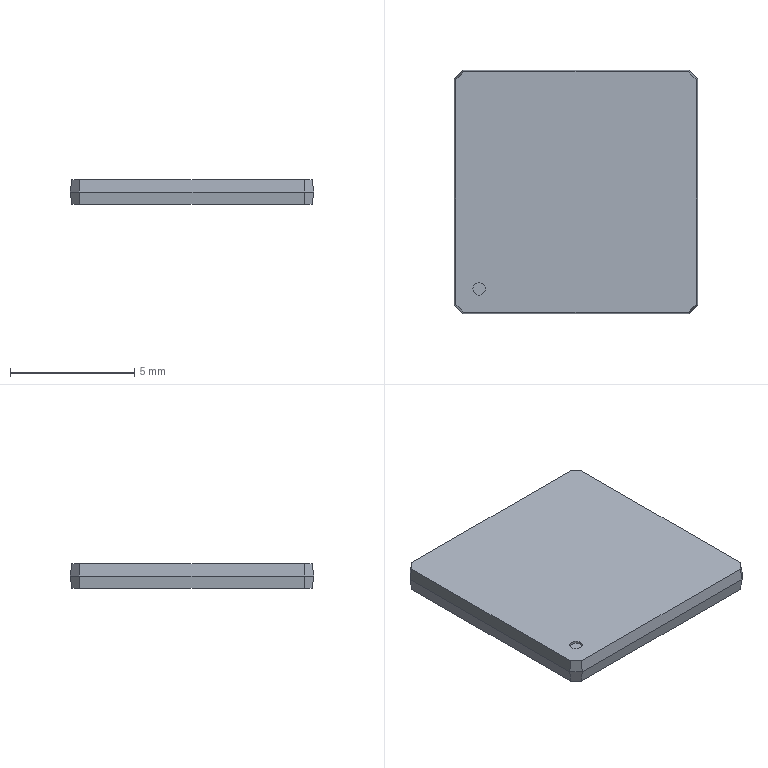Part | STEP file | RJ-USIO-V1_2-220411_260 | 1 solid | 21 faces | box 9.8 x 9.8 x 1 mm | volume 94.601 mm3 | plane 19 | cylinder 2 | commonest cylinder face diameters 0.5 x2
STEP:
#1=CARTESIAN_POINT('',(0.,0.,0.));
#2=DIRECTION('',(0.,0.,1.));
#3=DIRECTION('',(1.,0.,0.));
#4=AXIS2_PLACEMENT_3D('',#1,#2,#3);
#5=CARTESIAN_POINT('',(46.95,46.8,0.9));
#6=VERTEX_POINT('',#5);
#7=CARTESIAN_POINT('',(46.45,46.8,0.9));
#8=VERTEX_POINT('',#7);
#9=CARTESIAN_POINT('',(46.7,46.8,0.9));
#10=DIRECTION('',(0.,0.,1.));
#11=DIRECTION('',(1.,0.,0.));
#12=AXIS2_PLACEMENT_3D('',#9,#10,#11);
#13=CIRCLE('',#12,0.25);
#14=CARTESIAN_POINT('',(46.7,46.8,0.9));
#15=DIRECTION('',(0.,0.,1.));
#16=DIRECTION('',(-1.,0.,0.));
#17=AXIS2_PLACEMENT_3D('',#14,#15,#16);
#18=PLANE('',#17);
#19=CARTESIAN_POINT('',(0.,0.));
#20=DIRECTION('',(-1.,0.));
#21=AXIS2_PLACEMENT_2D('',#19,#20);
#22=CIRCLE('',#21,0.25);
#23=(GEOMETRIC_REPRESENTATION_CONTEXT(2)PARAMETRIC_REPRESENTATION_CONTEXT()REPRESENTATION_CONTEXT('',''));
#24=DEFINITIONAL_REPRESENTATION('',(#22),#23);
#25=PCURVE('',#18,#24);
#26=CARTESIAN_POINT('',(46.7,46.8,0.9));
#27=DIRECTION('',(0.,0.,1.));
#28=DIRECTION('',(-1.,0.,0.));
#29=AXIS2_PLACEMENT_3D('',#26,#27,#28);
#30=CYLINDRICAL_SURFACE('',#29,0.25);
#31=CARTESIAN_POINT('',(3.142,0.));
#32=DIRECTION('',(1.,0.));
#33=VECTOR('',#32,1.);
#34=LINE('',#31,#33);
#35=(GEOMETRIC_REPRESENTATION_CONTEXT(2)PARAMETRIC_REPRESENTATION_CONTEXT()REPRESENTATION_CONTEXT('',''));
#36=DEFINITIONAL_REPRESENTATION('',(#34),#35);
#37=PCURVE('',#30,#36);
#38=SURFACE_CURVE('',#13,(#25,#37),.PCURVE_S1.);
#39=EDGE_CURVE('',#6,#8,#38,.T.);
#40=ORIENTED_EDGE('',*,*,#39,.F.);
#41=CARTESIAN_POINT('',(46.7,46.8,0.9));
#42=DIRECTION('',(0.,0.,1.));
#43=DIRECTION('',(-1.,0.,0.));
#44=AXIS2_PLACEMENT_3D('',#41,#42,#43);
#45=CIRCLE('',#44,0.25);
#46=CARTESIAN_POINT('',(0.,0.));
#47=DIRECTION('',(1.,0.));
#48=AXIS2_PLACEMENT_2D('',#46,#47);
#49=CIRCLE('',#48,0.25);
#50=(GEOMETRIC_REPRESENTATION_CONTEXT(2)PARAMETRIC_REPRESENTATION_CONTEXT()REPRESENTATION_CONTEXT('',''));
#51=DEFINITIONAL_REPRESENTATION('',(#49),#50);
#52=PCURVE('',#18,#51);
#53=CARTESIAN_POINT('',(46.7,46.8,0.9));
#54=DIRECTION('',(0.,0.,1.));
#55=DIRECTION('',(-1.,0.,0.));
#56=AXIS2_PLACEMENT_3D('',#53,#54,#55);
#57=CYLINDRICAL_SURFACE('',#56,0.25);
#58=CARTESIAN_POINT('',(0.,0.));
#59=DIRECTION('',(1.,0.));
#60=VECTOR('',#59,1.);
#61=LINE('',#58,#60);
#62=(GEOMETRIC_REPRESENTATION_CONTEXT(2)PARAMETRIC_REPRESENTATION_CONTEXT()REPRESENTATION_CONTEXT('',''));
#63=DEFINITIONAL_REPRESENTATION('',(#61),#62);
#64=PCURVE('',#57,#63);
#65=SURFACE_CURVE('',#45,(#52,#64),.PCURVE_S1.);
#66=EDGE_CURVE('',#8,#6,#65,.T.);
#67=ORIENTED_EDGE('',*,*,#66,.F.);
#68=EDGE_LOOP('',(#40,#67));
#69=FACE_BOUND('',#68,.F.);
#70=ADVANCED_FACE('',(#69),#18,.T.);
#71=CARTESIAN_POINT('',(46.45,46.8,1.));
#72=VERTEX_POINT('',#71);
#73=CARTESIAN_POINT('',(46.45,46.8,0.9));
#74=DIRECTION('',(0.,0.,1.));
#75=VECTOR('',#74,1.);
#76=LINE('',#73,#75);
#77=CARTESIAN_POINT('',(6.283,0.));
#78=DIRECTION('',(0.,1.));
#79=VECTOR('',#78,1.);
#80=LINE('',#77,#79);
#81=(GEOMETRIC_REPRESENTATION_CONTEXT(2)PARAMETRIC_REPRESENTATION_CONTEXT()REPRESENTATION_CONTEXT('',''));
#82=DEFINITIONAL_REPRESENTATION('',(#80),#81);
#83=PCURVE('',#30,#82);
#84=CARTESIAN_POINT('',(0.,0.));
#85=DIRECTION('',(0.,1.));
#86=VECTOR('',#85,1.);
#87=LINE('',#84,#86);
#88=(GEOMETRIC_REPRESENTATION_CONTEXT(2)PARAMETRIC_REPRESENTATION_CONTEXT()REPRESENTATION_CONTEXT('',''));
#89=DEFINITIONAL_REPRESENTATION('',(#87),#88);
#90=PCURVE('',#57,#89);
#91=SURFACE_CURVE('',#76,(#83,#90),.PCURVE_S1.);
#92=EDGE_CURVE('',#8,#72,#91,.T.);
#93=ORIENTED_EDGE('',*,*,#92,.T.);
#94=CARTESIAN_POINT('',(46.95,46.8,1.));
#95=VERTEX_POINT('',#94);
#96=CARTESIAN_POINT('',(46.7,46.8,1.));
#97=DIRECTION('',(0.,0.,-1.));
#98=DIRECTION('',(-1.,0.,0.));
#99=AXIS2_PLACEMENT_3D('',#96,#97,#98);
#100=CIRCLE('',#99,0.25);
#101=CARTESIAN_POINT('',(6.283,0.1));
#102=DIRECTION('',(-1.,0.));
#103=VECTOR('',#102,1.);
#104=LINE('',#101,#103);
#105=(GEOMETRIC_REPRESENTATION_CONTEXT(2)PARAMETRIC_REPRESENTATION_CONTEXT()REPRESENTATION_CONTEXT('',''));
#106=DEFINITIONAL_REPRESENTATION('',(#104),#105);
#107=PCURVE('',#30,#106);
#108=CARTESIAN_POINT('',(45.7,45.8,1.));
#109=DIRECTION('',(0.,0.,1.));
#110=DIRECTION('',(-1.,0.,0.));
#111=AXIS2_PLACEMENT_3D('',#108,#109,#110);
#112=PLANE('',#111);
#113=CARTESIAN_POINT('',(-0.75,-1.));
#114=CARTESIAN_POINT('',(-0.75,-1.433));
#115=CARTESIAN_POINT('',(-1.125,-1.217));
#116=CARTESIAN_POINT('',(-1.5,-1.));
#117=CARTESIAN_POINT('',(-1.125,-0.7835));
#118=CARTESIAN_POINT('',(-0.75,-0.567));
#119=CARTESIAN_POINT('',(-0.75,-1.));
#120=(BOUNDED_CURVE()B_SPLINE_CURVE(2,(#113,#114,#115,#116,#117,#118,#119),.UNSPECIFIED.,.T.,.F.)B_SPLINE_CURVE_WITH_KNOTS((1,2,2,2,2,1),(-2.094,0.,2.094,4.189,6.283,8.378),.UNSPECIFIED.)CURVE()GEOMETRIC_REPRESENTATION_ITEM()RATIONAL_B_SPLINE_CURVE((1.,0.5,1.,0.5,1.,0.5,1.))REPRESENTATION_ITEM(''));
#121=(GEOMETRIC_REPRESENTATION_CONTEXT(2)PARAMETRIC_REPRESENTATION_CONTEXT()REPRESENTATION_CONTEXT('',''));
#122=DEFINITIONAL_REPRESENTATION('',(#120),#121);
#123=PCURVE('',#112,#122);
#124=SURFACE_CURVE('',#100,(#107,#123),.PCURVE_S1.);
#125=EDGE_CURVE('',#72,#95,#124,.T.);
#126=ORIENTED_EDGE('',*,*,#125,.T.);
#127=CARTESIAN_POINT('',(46.95,46.8,0.9));
#128=DIRECTION('',(0.,0.,1.));
#129=VECTOR('',#128,1.);
#130=LINE('',#127,#129);
#131=CARTESIAN_POINT('',(3.142,0.));
#132=DIRECTION('',(0.,1.));
#133=VECTOR('',#132,1.);
#134=LINE('',#131,#133);
#135=(GEOMETRIC_REPRESENTATION_CONTEXT(2)PARAMETRIC_REPRESENTATION_CONTEXT()REPRESENTATION_CONTEXT('',''));
#136=DEFINITIONAL_REPRESENTATION('',(#134),#135);
#137=PCURVE('',#30,#136);
#138=CARTESIAN_POINT('',(3.142,0.));
#139=DIRECTION('',(0.,1.));
#140=VECTOR('',#139,1.);
#141=LINE('',#138,#140);
#142=(GEOMETRIC_REPRESENTATION_CONTEXT(2)PARAMETRIC_REPRESENTATION_CONTEXT()REPRESENTATION_CONTEXT('',''));
#143=DEFINITIONAL_REPRESENTATION('',(#141),#142);
#144=PCURVE('',#57,#143);
#145=SURFACE_CURVE('',#130,(#137,#144),.PCURVE_S1.);
#146=EDGE_CURVE('',#6,#95,#145,.T.);
#147=ORIENTED_EDGE('',*,*,#146,.F.);
#148=ORIENTED_EDGE('',*,*,#39,.T.);
#149=EDGE_LOOP('',(#93,#126,#147,#148));
#150=FACE_BOUND('',#149,.F.);
#151=ADVANCED_FACE('',(#150),#30,.F.);
#152=ORIENTED_EDGE('',*,*,#66,.T.);
#153=ORIENTED_EDGE('',*,*,#146,.T.);
#154=CARTESIAN_POINT('',(46.7,46.8,1.));
#155=DIRECTION('',(0.,0.,-1.));
#156=DIRECTION('',(1.,0.,0.));
#157=AXIS2_PLACEMENT_3D('',#154,#155,#156);
#158=CIRCLE('',#157,0.25);
#159=CARTESIAN_POINT('',(3.142,0.1));
#160=DIRECTION('',(-1.,0.));
#161=VECTOR('',#160,1.);
#162=LINE('',#159,#161);
#163=(GEOMETRIC_REPRESENTATION_CONTEXT(2)PARAMETRIC_REPRESENTATION_CONTEXT()REPRESENTATION_CONTEXT('',''));
#164=DEFINITIONAL_REPRESENTATION('',(#162),#163);
#165=PCURVE('',#57,#164);
#166=CARTESIAN_POINT('',(-1.25,-1.));
#167=CARTESIAN_POINT('',(-1.25,-0.567));
#168=CARTESIAN_POINT('',(-0.875,-0.7835));
#169=CARTESIAN_POINT('',(-0.5,-1.));
#170=CARTESIAN_POINT('',(-0.875,-1.217));
#171=CARTESIAN_POINT('',(-1.25,-1.433));
#172=CARTESIAN_POINT('',(-1.25,-1.));
#173=(BOUNDED_CURVE()B_SPLINE_CURVE(2,(#166,#167,#168,#169,#170,#171,#172),.UNSPECIFIED.,.T.,.F.)B_SPLINE_CURVE_WITH_KNOTS((1,2,2,2,2,1),(-2.094,0.,2.094,4.189,6.283,8.378),.UNSPECIFIED.)CURVE()GEOMETRIC_REPRESENTATION_ITEM()RATIONAL_B_SPLINE_CURVE((1.,0.5,1.,0.5,1.,0.5,1.))REPRESENTATION_ITEM(''));
#174=(GEOMETRIC_REPRESENTATION_CONTEXT(2)PARAMETRIC_REPRESENTATION_CONTEXT()REPRESENTATION_CONTEXT('',''));
#175=DEFINITIONAL_REPRESENTATION('',(#173),#174);
#176=PCURVE('',#112,#175);
#177=SURFACE_CURVE('',#158,(#165,#176),.PCURVE_S1.);
#178=EDGE_CURVE('',#95,#72,#177,.T.);
#179=ORIENTED_EDGE('',*,*,#178,.T.);
#180=ORIENTED_EDGE('',*,*,#92,.F.);
#181=EDGE_LOOP('',(#152,#153,#179,#180));
#182=FACE_BOUND('',#181,.F.);
#183=ADVANCED_FACE('',(#182),#57,.F.);
#184=CARTESIAN_POINT('',(55.439,55.225,1.));
#185=VERTEX_POINT('',#184);
#186=CARTESIAN_POINT('',(55.439,46.175,1.));
#187=VERTEX_POINT('',#186);
#188=CARTESIAN_POINT('',(55.439,55.225,1.));
#189=DIRECTION('',(0.,-1.,0.));
#190=VECTOR('',#189,1.);
#191=LINE('',#188,#190);
#192=CARTESIAN_POINT('',(-9.739,-9.425));
#193=DIRECTION('',(0.,1.));
#194=VECTOR('',#193,1.);
#195=LINE('',#192,#194);
#196=(GEOMETRIC_REPRESENTATION_CONTEXT(2)PARAMETRIC_REPRESENTATION_CONTEXT()REPRESENTATION_CONTEXT('',''));
#197=DEFINITIONAL_REPRESENTATION('',(#195),#196);
#198=PCURVE('',#112,#197);
#199=CARTESIAN_POINT('',(55.439,45.8,1.));
#200=DIRECTION('',(0.9925,0.,0.1219));
#201=DIRECTION('',(-0.1219,0.,0.9925));
#202=AXIS2_PLACEMENT_3D('',#199,#200,#201);
#203=PLANE('',#202);
#204=CARTESIAN_POINT('',(0.,-9.425));
#205=DIRECTION('',(0.,1.));
#206=VECTOR('',#205,1.);
#207=LINE('',#204,#206);
#208=(GEOMETRIC_REPRESENTATION_CONTEXT(2)PARAMETRIC_REPRESENTATION_CONTEXT()REPRESENTATION_CONTEXT('',''));
#209=DEFINITIONAL_REPRESENTATION('',(#207),#208);
#210=PCURVE('',#203,#209);
#211=SURFACE_CURVE('',#191,(#198,#210),.PCURVE_S1.);
#212=EDGE_CURVE('',#185,#187,#211,.T.);
#213=ORIENTED_EDGE('',*,*,#212,.T.);
#214=CARTESIAN_POINT('',(55.125,45.861,1.));
#215=VERTEX_POINT('',#214);
#216=CARTESIAN_POINT('',(55.125,45.861,1.));
#217=DIRECTION('',(0.7071,0.7071,0.));
#218=VECTOR('',#217,1.);
#219=LINE('',#216,#218);
#220=CARTESIAN_POINT('',(-9.425,-0.06139));
#221=DIRECTION('',(-0.7071,-0.7071));
#222=VECTOR('',#221,1.);
#223=LINE('',#220,#222);
#224=(GEOMETRIC_REPRESENTATION_CONTEXT(2)PARAMETRIC_REPRESENTATION_CONTEXT()REPRESENTATION_CONTEXT('',''));
#225=DEFINITIONAL_REPRESENTATION('',(#223),#224);
#226=PCURVE('',#112,#225);
#227=CARTESIAN_POINT('',(50.382,41.118,1.));
#228=DIRECTION('',(0.7018,-0.7018,0.1219));
#229=DIRECTION('',(-0.7071,-0.7071,0.));
#230=AXIS2_PLACEMENT_3D('',#227,#228,#229);
#231=PLANE('',#230);
#232=CARTESIAN_POINT('',(-6.708,0.));
#233=DIRECTION('',(-1.,0.));
#234=VECTOR('',#233,1.);
#235=LINE('',#232,#234);
#236=(GEOMETRIC_REPRESENTATION_CONTEXT(2)PARAMETRIC_REPRESENTATION_CONTEXT()REPRESENTATION_CONTEXT('',''));
#237=DEFINITIONAL_REPRESENTATION('',(#235),#236);
#238=PCURVE('',#231,#237);
#239=SURFACE_CURVE('',#219,(#226,#238),.PCURVE_S1.);
#240=EDGE_CURVE('',#215,#187,#239,.T.);
#241=ORIENTED_EDGE('',*,*,#240,.F.);
#242=CARTESIAN_POINT('',(46.075,45.861,1.));
#243=VERTEX_POINT('',#242);
#244=CARTESIAN_POINT('',(55.125,45.861,1.));
#245=DIRECTION('',(-1.,0.,0.));
#246=VECTOR('',#245,1.);
#247=LINE('',#244,#246);
#248=CARTESIAN_POINT('',(-9.425,-0.06139));
#249=DIRECTION('',(1.,0.));
#250=VECTOR('',#249,1.);
#251=LINE('',#248,#250);
#252=(GEOMETRIC_REPRESENTATION_CONTEXT(2)PARAMETRIC_REPRESENTATION_CONTEXT()REPRESENTATION_CONTEXT('',''));
#253=DEFINITIONAL_REPRESENTATION('',(#251),#252);
#254=PCURVE('',#112,#253);
#255=CARTESIAN_POINT('',(45.7,45.861,1.));
#256=DIRECTION('',(0.,-0.9925,0.1219));
#257=DIRECTION('',(0.,0.1219,0.9925));
#258=AXIS2_PLACEMENT_3D('',#255,#256,#257);
#259=PLANE('',#258);
#260=CARTESIAN_POINT('',(0.,-9.425));
#261=DIRECTION('',(0.,1.));
#262=VECTOR('',#261,1.);
#263=LINE('',#260,#262);
#264=(GEOMETRIC_REPRESENTATION_CONTEXT(2)PARAMETRIC_REPRESENTATION_CONTEXT()REPRESENTATION_CONTEXT('',''));
#265=DEFINITIONAL_REPRESENTATION('',(#263),#264);
#266=PCURVE('',#259,#265);
#267=SURFACE_CURVE('',#247,(#254,#266),.PCURVE_S1.);
#268=EDGE_CURVE('',#215,#243,#267,.T.);
#269=ORIENTED_EDGE('',*,*,#268,.T.);
#270=CARTESIAN_POINT('',(45.761,46.175,1.));
#271=VERTEX_POINT('',#270);
#272=CARTESIAN_POINT('',(45.761,46.175,1.));
#273=DIRECTION('',(0.7071,-0.7071,0.));
#274=VECTOR('',#273,1.);
#275=LINE('',#272,#274);
#276=CARTESIAN_POINT('',(-0.06139,-0.3754));
#277=DIRECTION('',(-0.7071,0.7071));
#278=VECTOR('',#277,1.);
#279=LINE('',#276,#278);
#280=(GEOMETRIC_REPRESENTATION_CONTEXT(2)PARAMETRIC_REPRESENTATION_CONTEXT()REPRESENTATION_CONTEXT('',''));
#281=DEFINITIONAL_REPRESENTATION('',(#279),#280);
#282=PCURVE('',#112,#281);
#283=CARTESIAN_POINT('',(45.918,46.018,1.));
#284=DIRECTION('',(-0.7018,-0.7018,0.1219));
#285=DIRECTION('',(-0.7071,0.7071,0.));
#286=AXIS2_PLACEMENT_3D('',#283,#284,#285);
#287=PLANE('',#286);
#288=CARTESIAN_POINT('',(0.2221,0.));
#289=DIRECTION('',(-1.,0.));
#290=VECTOR('',#289,1.);
#291=LINE('',#288,#290);
#292=(GEOMETRIC_REPRESENTATION_CONTEXT(2)PARAMETRIC_REPRESENTATION_CONTEXT()REPRESENTATION_CONTEXT('',''));
#293=DEFINITIONAL_REPRESENTATION('',(#291),#292);
#294=PCURVE('',#287,#293);
#295=SURFACE_CURVE('',#275,(#282,#294),.PCURVE_S1.);
#296=EDGE_CURVE('',#271,#243,#295,.T.);
#297=ORIENTED_EDGE('',*,*,#296,.F.);
#298=CARTESIAN_POINT('',(45.761,55.225,1.));
#299=VERTEX_POINT('',#298);
#300=CARTESIAN_POINT('',(45.761,46.175,1.));
#301=DIRECTION('',(0.,1.,0.));
#302=VECTOR('',#301,1.);
#303=LINE('',#300,#302);
#304=CARTESIAN_POINT('',(-0.06139,-0.3754));
#305=DIRECTION('',(0.,-1.));
#306=VECTOR('',#305,1.);
#307=LINE('',#304,#306);
#308=(GEOMETRIC_REPRESENTATION_CONTEXT(2)PARAMETRIC_REPRESENTATION_CONTEXT()REPRESENTATION_CONTEXT('',''));
#309=DEFINITIONAL_REPRESENTATION('',(#307),#308);
#310=PCURVE('',#112,#309);
#311=CARTESIAN_POINT('',(45.761,45.8,1.));
#312=DIRECTION('',(-0.9925,0.,0.1219));
#313=DIRECTION('',(-0.1219,0.,-0.9925));
#314=AXIS2_PLACEMENT_3D('',#311,#312,#313);
#315=PLANE('',#314);
#316=CARTESIAN_POINT('',(0.,-0.3754));
#317=DIRECTION('',(0.,-1.));
#318=VECTOR('',#317,1.);
#319=LINE('',#316,#318);
#320=(GEOMETRIC_REPRESENTATION_CONTEXT(2)PARAMETRIC_REPRESENTATION_CONTEXT()REPRESENTATION_CONTEXT('',''));
#321=DEFINITIONAL_REPRESENTATION('',(#319),#320);
#322=PCURVE('',#315,#321);
#323=SURFACE_CURVE('',#303,(#310,#322),.PCURVE_S1.);
#324=EDGE_CURVE('',#271,#299,#323,.T.);
#325=ORIENTED_EDGE('',*,*,#324,.T.);
#326=CARTESIAN_POINT('',(46.075,55.539,1.));
#327=VERTEX_POINT('',#326);
#328=CARTESIAN_POINT('',(46.075,55.539,1.));
#329=DIRECTION('',(-0.7071,-0.7071,0.));
#330=VECTOR('',#329,1.);
#331=LINE('',#328,#330);
#332=CARTESIAN_POINT('',(-0.3754,-9.739));
#333=DIRECTION('',(0.7071,0.7071));
#334=VECTOR('',#333,1.);
#335=LINE('',#332,#334);
#336=(GEOMETRIC_REPRESENTATION_CONTEXT(2)PARAMETRIC_REPRESENTATION_CONTEXT()REPRESENTATION_CONTEXT('',''));
#337=DEFINITIONAL_REPRESENTATION('',(#335),#336);
#338=PCURVE('',#112,#337);
#339=CARTESIAN_POINT('',(41.018,50.482,1.));
#340=DIRECTION('',(-0.7018,0.7018,0.1219));
#341=DIRECTION('',(0.7071,0.7071,0.));
#342=AXIS2_PLACEMENT_3D('',#339,#340,#341);
#343=PLANE('',#342);
#344=CARTESIAN_POINT('',(7.152,0.));
#345=DIRECTION('',(-1.,0.));
#346=VECTOR('',#345,1.);
#347=LINE('',#344,#346);
#348=(GEOMETRIC_REPRESENTATION_CONTEXT(2)PARAMETRIC_REPRESENTATION_CONTEXT()REPRESENTATION_CONTEXT('',''));
#349=DEFINITIONAL_REPRESENTATION('',(#347),#348);
#350=PCURVE('',#343,#349);
#351=SURFACE_CURVE('',#331,(#338,#350),.PCURVE_S1.);
#352=EDGE_CURVE('',#327,#299,#351,.T.);
#353=ORIENTED_EDGE('',*,*,#352,.F.);
#354=CARTESIAN_POINT('',(55.125,55.539,1.));
#355=VERTEX_POINT('',#354);
#356=CARTESIAN_POINT('',(46.075,55.539,1.));
#357=DIRECTION('',(1.,0.,0.));
#358=VECTOR('',#357,1.);
#359=LINE('',#356,#358);
#360=CARTESIAN_POINT('',(-0.3754,-9.739));
#361=DIRECTION('',(-1.,0.));
#362=VECTOR('',#361,1.);
#363=LINE('',#360,#362);
#364=(GEOMETRIC_REPRESENTATION_CONTEXT(2)PARAMETRIC_REPRESENTATION_CONTEXT()REPRESENTATION_CONTEXT('',''));
#365=DEFINITIONAL_REPRESENTATION('',(#363),#364);
#366=PCURVE('',#112,#365);
#367=CARTESIAN_POINT('',(45.7,55.539,1.));
#368=DIRECTION('',(0.,0.9925,0.1219));
#369=DIRECTION('',(0.,0.1219,-0.9925));
#370=AXIS2_PLACEMENT_3D('',#367,#368,#369);
#371=PLANE('',#370);
#372=CARTESIAN_POINT('',(0.,-0.3754));
#373=DIRECTION('',(0.,-1.));
#374=VECTOR('',#373,1.);
#375=LINE('',#372,#374);
#376=(GEOMETRIC_REPRESENTATION_CONTEXT(2)PARAMETRIC_REPRESENTATION_CONTEXT()REPRESENTATION_CONTEXT('',''));
#377=DEFINITIONAL_REPRESENTATION('',(#375),#376);
#378=PCURVE('',#371,#377);
#379=SURFACE_CURVE('',#359,(#366,#378),.PCURVE_S1.);
#380=EDGE_CURVE('',#327,#355,#379,.T.);
#381=ORIENTED_EDGE('',*,*,#380,.T.);
#382=CARTESIAN_POINT('',(55.439,55.225,1.));
#383=DIRECTION('',(-0.7071,0.7071,0.));
#384=VECTOR('',#383,1.);
#385=LINE('',#382,#384);
#386=CARTESIAN_POINT('',(-9.739,-9.425));
#387=DIRECTION('',(0.7071,-0.7071));
#388=VECTOR('',#387,1.);
#389=LINE('',#386,#388);
#390=(GEOMETRIC_REPRESENTATION_CONTEXT(2)PARAMETRIC_REPRESENTATION_CONTEXT()REPRESENTATION_CONTEXT('',''));
#391=DEFINITIONAL_REPRESENTATION('',(#389),#390);
#392=PCURVE('',#112,#391);
#393=CARTESIAN_POINT('',(55.282,55.382,1.));
#394=DIRECTION('',(0.7018,0.7018,0.1219));
#395=DIRECTION('',(0.7071,-0.7071,0.));
#396=AXIS2_PLACEMENT_3D('',#393,#394,#395);
#397=PLANE('',#396);
#398=CARTESIAN_POINT('',(0.2221,0.));
#399=DIRECTION('',(-1.,0.));
#400=VECTOR('',#399,1.);
#401=LINE('',#398,#400);
#402=(GEOMETRIC_REPRESENTATION_CONTEXT(2)PARAMETRIC_REPRESENTATION_CONTEXT()REPRESENTATION_CONTEXT('',''));
#403=DEFINITIONAL_REPRESENTATION('',(#401),#402);
#404=PCURVE('',#397,#403);
#405=SURFACE_CURVE('',#385,(#392,#404),.PCURVE_S1.);
#406=EDGE_CURVE('',#185,#355,#405,.T.);
#407=ORIENTED_EDGE('',*,*,#406,.F.);
#408=EDGE_LOOP('',(#213,#241,#269,#297,#325,#353,#381,#407));
#409=FACE_BOUND('',#408,.F.);
#410=ORIENTED_EDGE('',*,*,#125,.F.);
#411=ORIENTED_EDGE('',*,*,#178,.F.);
#412=EDGE_LOOP('',(#410,#411));
#413=FACE_BOUND('',#412,.F.);
#414=ADVANCED_FACE('',(#409,#413),#112,.T.);
#415=CARTESIAN_POINT('',(55.5,46.15,0.5));
#416=VERTEX_POINT('',#415);
#417=CARTESIAN_POINT('',(55.5,46.15,0.5));
#418=DIRECTION('',(-0.1217,0.05042,0.9913));
#419=VECTOR('',#418,1.);
#420=LINE('',#417,#419);
#421=CARTESIAN_POINT('',(-0.5038,-0.35));
#422=DIRECTION('',(0.9987,-0.05042));
#423=VECTOR('',#422,1.);
#424=LINE('',#421,#423);
#425=(GEOMETRIC_REPRESENTATION_CONTEXT(2)PARAMETRIC_REPRESENTATION_CONTEXT()REPRESENTATION_CONTEXT('',''));
#426=DEFINITIONAL_REPRESENTATION('',(#424),#425);
#427=PCURVE('',#203,#426);
#428=CARTESIAN_POINT('',(-7.177,0.5038));
#429=DIRECTION('',(0.05042,-0.9987));
#430=VECTOR('',#429,1.);
#431=LINE('',#428,#430);
#432=(GEOMETRIC_REPRESENTATION_CONTEXT(2)PARAMETRIC_REPRESENTATION_CONTEXT()REPRESENTATION_CONTEXT('',''));
#433=DEFINITIONAL_REPRESENTATION('',(#431),#432);
#434=PCURVE('',#231,#433);
#435=SURFACE_CURVE('',#420,(#427,#434),.PCURVE_S1.);
#436=EDGE_CURVE('',#416,#187,#435,.T.);
#437=ORIENTED_EDGE('',*,*,#436,.T.);
#438=ORIENTED_EDGE('',*,*,#212,.F.);
#439=CARTESIAN_POINT('',(55.5,55.25,0.5));
#440=VERTEX_POINT('',#439);
#441=CARTESIAN_POINT('',(55.5,55.25,0.5));
#442=DIRECTION('',(-0.1217,-0.05042,0.9913));
#443=VECTOR('',#442,1.);
#444=LINE('',#441,#443);
#445=CARTESIAN_POINT('',(-0.5038,-9.45));
#446=DIRECTION('',(0.9987,0.05042));
#447=VECTOR('',#446,1.);
#448=LINE('',#445,#447);
#449=(GEOMETRIC_REPRESENTATION_CONTEXT(2)PARAMETRIC_REPRESENTATION_CONTEXT()REPRESENTATION_CONTEXT('',''));
#450=DEFINITIONAL_REPRESENTATION('',(#448),#449);
#451=PCURVE('',#203,#450);
#452=CARTESIAN_POINT('',(0.2475,0.5038));
#453=DIRECTION('',(-0.05042,-0.9987));
#454=VECTOR('',#453,1.);
#455=LINE('',#452,#454);
#456=(GEOMETRIC_REPRESENTATION_CONTEXT(2)PARAMETRIC_REPRESENTATION_CONTEXT()REPRESENTATION_CONTEXT('',''));
#457=DEFINITIONAL_REPRESENTATION('',(#455),#456);
#458=PCURVE('',#397,#457);
#459=SURFACE_CURVE('',#444,(#451,#458),.PCURVE_S1.);
#460=EDGE_CURVE('',#440,#185,#459,.T.);
#461=ORIENTED_EDGE('',*,*,#460,.F.);
#462=CARTESIAN_POINT('',(55.5,46.15,0.5));
#463=DIRECTION('',(0.,1.,0.));
#464=VECTOR('',#463,1.);
#465=LINE('',#462,#464);
#466=CARTESIAN_POINT('',(-0.5038,-0.35));
#467=DIRECTION('',(0.,-1.));
#468=VECTOR('',#467,1.);
#469=LINE('',#466,#468);
#470=(GEOMETRIC_REPRESENTATION_CONTEXT(2)PARAMETRIC_REPRESENTATION_CONTEXT()REPRESENTATION_CONTEXT('',''));
#471=DEFINITIONAL_REPRESENTATION('',(#469),#470);
#472=PCURVE('',#203,#471);
#473=CARTESIAN_POINT('',(55.5,55.25,0.5));
#474=DIRECTION('',(-0.9925,0.,0.1219));
#475=DIRECTION('',(-0.1219,0.,-0.9925));
#476=AXIS2_PLACEMENT_3D('',#473,#474,#475);
#477=PLANE('',#476);
#478=CARTESIAN_POINT('',(0.,9.1));
#479=DIRECTION('',(0.,-1.));
#480=VECTOR('',#479,1.);
#481=LINE('',#478,#480);
#482=(GEOMETRIC_REPRESENTATION_CONTEXT(2)PARAMETRIC_REPRESENTATION_CONTEXT()REPRESENTATION_CONTEXT('',''));
#483=DEFINITIONAL_REPRESENTATION('',(#481),#482);
#484=PCURVE('',#477,#483);
#485=SURFACE_CURVE('',#465,(#472,#484),.PCURVE_S1.);
#486=EDGE_CURVE('',#416,#440,#485,.T.);
#487=ORIENTED_EDGE('',*,*,#486,.F.);
#488=EDGE_LOOP('',(#437,#438,#461,#487));
#489=FACE_BOUND('',#488,.F.);
#490=ADVANCED_FACE('',(#489),#203,.T.);
#491=CARTESIAN_POINT('',(55.15,45.8,0.5));
#492=VERTEX_POINT('',#491);
#493=CARTESIAN_POINT('',(55.15,45.8,0.5));
#494=DIRECTION('',(-0.05042,0.1217,0.9913));
#495=VECTOR('',#494,1.);
#496=LINE('',#493,#495);
#497=CARTESIAN_POINT('',(-6.682,0.5038));
#498=DIRECTION('',(-0.05042,-0.9987));
#499=VECTOR('',#498,1.);
#500=LINE('',#497,#499);
#501=(GEOMETRIC_REPRESENTATION_CONTEXT(2)PARAMETRIC_REPRESENTATION_CONTEXT()REPRESENTATION_CONTEXT('',''));
#502=DEFINITIONAL_REPRESENTATION('',(#500),#501);
#503=PCURVE('',#231,#502);
#504=CARTESIAN_POINT('',(-0.5038,-9.45));
#505=DIRECTION('',(0.9987,0.05042));
#506=VECTOR('',#505,1.);
#507=LINE('',#504,#506);
#508=(GEOMETRIC_REPRESENTATION_CONTEXT(2)PARAMETRIC_REPRESENTATION_CONTEXT()REPRESENTATION_CONTEXT('',''));
#509=DEFINITIONAL_REPRESENTATION('',(#507),#508);
#510=PCURVE('',#259,#509);
#511=SURFACE_CURVE('',#496,(#503,#510),.PCURVE_S1.);
#512=EDGE_CURVE('',#492,#215,#511,.T.);
#513=ORIENTED_EDGE('',*,*,#512,.T.);
#514=ORIENTED_EDGE('',*,*,#240,.T.);
#515=ORIENTED_EDGE('',*,*,#436,.F.);
#516=CARTESIAN_POINT('',(55.15,45.8,0.5));
#517=DIRECTION('',(0.7071,0.7071,0.));
#518=VECTOR('',#517,1.);
#519=LINE('',#516,#518);
#520=CARTESIAN_POINT('',(-6.682,0.5038));
#521=DIRECTION('',(-1.,0.));
#522=VECTOR('',#521,1.);
#523=LINE('',#520,#522);
#524=(GEOMETRIC_REPRESENTATION_CONTEXT(2)PARAMETRIC_REPRESENTATION_CONTEXT()REPRESENTATION_CONTEXT('',''));
#525=DEFINITIONAL_REPRESENTATION('',(#523),#524);
#526=PCURVE('',#231,#525);
#527=CARTESIAN_POINT('',(55.15,45.8,0.5));
#528=DIRECTION('',(-0.7018,0.7018,0.1219));
#529=DIRECTION('',(0.7071,0.7071,0.));
#530=AXIS2_PLACEMENT_3D('',#527,#528,#529);
#531=PLANE('',#530);
#532=CARTESIAN_POINT('',(0.,0.));
#533=DIRECTION('',(1.,0.));
#534=VECTOR('',#533,1.);
#535=LINE('',#532,#534);
#536=(GEOMETRIC_REPRESENTATION_CONTEXT(2)PARAMETRIC_REPRESENTATION_CONTEXT()REPRESENTATION_CONTEXT('',''));
#537=DEFINITIONAL_REPRESENTATION('',(#535),#536);
#538=PCURVE('',#531,#537);
#539=SURFACE_CURVE('',#519,(#526,#538),.PCURVE_S1.);
#540=EDGE_CURVE('',#492,#416,#539,.T.);
#541=ORIENTED_EDGE('',*,*,#540,.F.);
#542=EDGE_LOOP('',(#513,#514,#515,#541));
#543=FACE_BOUND('',#542,.F.);
#544=ADVANCED_FACE('',(#543),#231,.T.);
#545=CARTESIAN_POINT('',(46.05,45.8,0.5));
#546=VERTEX_POINT('',#545);
#547=CARTESIAN_POINT('',(46.05,45.8,0.5));
#548=DIRECTION('',(0.05042,0.1217,0.9913));
#549=VECTOR('',#548,1.);
#550=LINE('',#547,#549);
#551=CARTESIAN_POINT('',(-0.5038,-0.35));
#552=DIRECTION('',(0.9987,-0.05042));
#553=VECTOR('',#552,1.);
#554=LINE('',#551,#553);
#555=(GEOMETRIC_REPRESENTATION_CONTEXT(2)PARAMETRIC_REPRESENTATION_CONTEXT()REPRESENTATION_CONTEXT('',''));
#556=DEFINITIONAL_REPRESENTATION('',(#554),#555);
#557=PCURVE('',#259,#556);
#558=CARTESIAN_POINT('',(-0.2475,0.5038));
#559=DIRECTION('',(0.05042,-0.9987));
#560=VECTOR('',#559,1.);
#561=LINE('',#558,#560);
#562=(GEOMETRIC_REPRESENTATION_CONTEXT(2)PARAMETRIC_REPRESENTATION_CONTEXT()REPRESENTATION_CONTEXT('',''));
#563=DEFINITIONAL_REPRESENTATION('',(#561),#562);
#564=PCURVE('',#287,#563);
#565=SURFACE_CURVE('',#550,(#557,#564),.PCURVE_S1.);
#566=EDGE_CURVE('',#546,#243,#565,.T.);
#567=ORIENTED_EDGE('',*,*,#566,.T.);
#568=ORIENTED_EDGE('',*,*,#268,.F.);
#569=ORIENTED_EDGE('',*,*,#512,.F.);
#570=CARTESIAN_POINT('',(46.05,45.8,0.5));
#571=DIRECTION('',(1.,0.,0.));
#572=VECTOR('',#571,1.);
#573=LINE('',#570,#572);
#574=CARTESIAN_POINT('',(-0.5038,-0.35));
#575=DIRECTION('',(0.,-1.));
#576=VECTOR('',#575,1.);
#577=LINE('',#574,#576);
#578=(GEOMETRIC_REPRESENTATION_CONTEXT(2)PARAMETRIC_REPRESENTATION_CONTEXT()REPRESENTATION_CONTEXT('',''));
#579=DEFINITIONAL_REPRESENTATION('',(#577),#578);
#580=PCURVE('',#259,#579);
#581=CARTESIAN_POINT('',(46.05,45.8,0.5));
#582=DIRECTION('',(0.,0.9925,0.1219));
#583=DIRECTION('',(0.,0.1219,-0.9925));
#584=AXIS2_PLACEMENT_3D('',#581,#582,#583);
#585=PLANE('',#584);
#586=CARTESIAN_POINT('',(0.,0.));
#587=DIRECTION('',(0.,-1.));
#588=VECTOR('',#587,1.);
#589=LINE('',#586,#588);
#590=(GEOMETRIC_REPRESENTATION_CONTEXT(2)PARAMETRIC_REPRESENTATION_CONTEXT()REPRESENTATION_CONTEXT('',''));
#591=DEFINITIONAL_REPRESENTATION('',(#589),#590);
#592=PCURVE('',#585,#591);
#593=SURFACE_CURVE('',#573,(#580,#592),.PCURVE_S1.);
#594=EDGE_CURVE('',#546,#492,#593,.T.);
#595=ORIENTED_EDGE('',*,*,#594,.F.);
#596=EDGE_LOOP('',(#567,#568,#569,#595));
#597=FACE_BOUND('',#596,.F.);
#598=ADVANCED_FACE('',(#597),#259,.T.);
#599=CARTESIAN_POINT('',(45.7,46.15,0.5));
#600=VERTEX_POINT('',#599);
#601=CARTESIAN_POINT('',(45.761,46.175,1.));
#602=DIRECTION('',(-0.1217,-0.05042,-0.9913));
#603=VECTOR('',#602,1.);
#604=LINE('',#601,#603);
#605=CARTESIAN_POINT('',(0.2221,0.));
#606=DIRECTION('',(0.05042,0.9987));
#607=VECTOR('',#606,1.);
#608=LINE('',#605,#607);
#609=(GEOMETRIC_REPRESENTATION_CONTEXT(2)PARAMETRIC_REPRESENTATION_CONTEXT()REPRESENTATION_CONTEXT('',''));
#610=DEFINITIONAL_REPRESENTATION('',(#608),#609);
#611=PCURVE('',#287,#610);
#612=CARTESIAN_POINT('',(0.,-0.3754));
#613=DIRECTION('',(0.9987,0.05042));
#614=VECTOR('',#613,1.);
#615=LINE('',#612,#614);
#616=(GEOMETRIC_REPRESENTATION_CONTEXT(2)PARAMETRIC_REPRESENTATION_CONTEXT()REPRESENTATION_CONTEXT('',''));
#617=DEFINITIONAL_REPRESENTATION('',(#615),#616);
#618=PCURVE('',#315,#617);
#619=SURFACE_CURVE('',#604,(#611,#618),.PCURVE_S1.);
#620=EDGE_CURVE('',#271,#600,#619,.T.);
#621=ORIENTED_EDGE('',*,*,#620,.F.);
#622=ORIENTED_EDGE('',*,*,#296,.T.);
#623=ORIENTED_EDGE('',*,*,#566,.F.);
#624=CARTESIAN_POINT('',(45.7,46.15,0.5));
#625=DIRECTION('',(0.7071,-0.7071,0.));
#626=VECTOR('',#625,1.);
#627=LINE('',#624,#626);
#628=CARTESIAN_POINT('',(0.2475,0.5038));
#629=DIRECTION('',(-1.,0.));
#630=VECTOR('',#629,1.);
#631=LINE('',#628,#630);
#632=(GEOMETRIC_REPRESENTATION_CONTEXT(2)PARAMETRIC_REPRESENTATION_CONTEXT()REPRESENTATION_CONTEXT('',''));
#633=DEFINITIONAL_REPRESENTATION('',(#631),#632);
#634=PCURVE('',#287,#633);
#635=CARTESIAN_POINT('',(45.7,46.15,0.5));
#636=DIRECTION('',(0.7018,0.7018,0.1219));
#637=DIRECTION('',(0.7071,-0.7071,0.));
#638=AXIS2_PLACEMENT_3D('',#635,#636,#637);
#639=PLANE('',#638);
#640=CARTESIAN_POINT('',(0.,0.));
#641=DIRECTION('',(1.,0.));
#642=VECTOR('',#641,1.);
#643=LINE('',#640,#642);
#644=(GEOMETRIC_REPRESENTATION_CONTEXT(2)PARAMETRIC_REPRESENTATION_CONTEXT()REPRESENTATION_CONTEXT('',''));
#645=DEFINITIONAL_REPRESENTATION('',(#643),#644);
#646=PCURVE('',#639,#645);
#647=SURFACE_CURVE('',#627,(#634,#646),.PCURVE_S1.);
#648=EDGE_CURVE('',#600,#546,#647,.T.);
#649=ORIENTED_EDGE('',*,*,#648,.F.);
#650=EDGE_LOOP('',(#621,#622,#623,#649));
#651=FACE_BOUND('',#650,.F.);
#652=ADVANCED_FACE('',(#651),#287,.T.);
#653=ORIENTED_EDGE('',*,*,#620,.T.);
#654=CARTESIAN_POINT('',(45.7,55.25,0.5));
#655=VERTEX_POINT('',#654);
#656=CARTESIAN_POINT('',(45.7,55.25,0.5));
#657=DIRECTION('',(0.,-1.,0.));
#658=VECTOR('',#657,1.);
#659=LINE('',#656,#658);
#660=CARTESIAN_POINT('',(0.5038,-9.45));
#661=DIRECTION('',(0.,1.));
#662=VECTOR('',#661,1.);
#663=LINE('',#660,#662);
#664=(GEOMETRIC_REPRESENTATION_CONTEXT(2)PARAMETRIC_REPRESENTATION_CONTEXT()REPRESENTATION_CONTEXT('',''));
#665=DEFINITIONAL_REPRESENTATION('',(#663),#664);
#666=PCURVE('',#315,#665);
#667=CARTESIAN_POINT('',(45.7,55.25,0.5));
#668=DIRECTION('',(0.9925,0.,0.1219));
#669=DIRECTION('',(-0.1219,0.,0.9925));
#670=AXIS2_PLACEMENT_3D('',#667,#668,#669);
#671=PLANE('',#670);
#672=CARTESIAN_POINT('',(0.,0.));
#673=DIRECTION('',(0.,1.));
#674=VECTOR('',#673,1.);
#675=LINE('',#672,#674);
#676=(GEOMETRIC_REPRESENTATION_CONTEXT(2)PARAMETRIC_REPRESENTATION_CONTEXT()REPRESENTATION_CONTEXT('',''));
#677=DEFINITIONAL_REPRESENTATION('',(#675),#676);
#678=PCURVE('',#671,#677);
#679=SURFACE_CURVE('',#659,(#666,#678),.PCURVE_S1.);
#680=EDGE_CURVE('',#655,#600,#679,.T.);
#681=ORIENTED_EDGE('',*,*,#680,.F.);
#682=CARTESIAN_POINT('',(45.761,55.225,1.));
#683=DIRECTION('',(-0.1217,0.05042,-0.9913));
#684=VECTOR('',#683,1.);
#685=LINE('',#682,#684);
#686=CARTESIAN_POINT('',(0.,-9.425));
#687=DIRECTION('',(0.9987,-0.05042));
#688=VECTOR('',#687,1.);
#689=LINE('',#686,#688);
#690=(GEOMETRIC_REPRESENTATION_CONTEXT(2)PARAMETRIC_REPRESENTATION_CONTEXT()REPRESENTATION_CONTEXT('',''));
#691=DEFINITIONAL_REPRESENTATION('',(#689),#690);
#692=PCURVE('',#315,#691);
#693=CARTESIAN_POINT('',(6.708,0.));
#694=DIRECTION('',(-0.05042,0.9987));
#695=VECTOR('',#694,1.);
#696=LINE('',#693,#695);
#697=(GEOMETRIC_REPRESENTATION_CONTEXT(2)PARAMETRIC_REPRESENTATION_CONTEXT()REPRESENTATION_CONTEXT('',''));
#698=DEFINITIONAL_REPRESENTATION('',(#696),#697);
#699=PCURVE('',#343,#698);
#700=SURFACE_CURVE('',#685,(#692,#699),.PCURVE_S1.);
#701=EDGE_CURVE('',#299,#655,#700,.T.);
#702=ORIENTED_EDGE('',*,*,#701,.F.);
#703=ORIENTED_EDGE('',*,*,#324,.F.);
#704=EDGE_LOOP('',(#653,#681,#702,#703));
#705=FACE_BOUND('',#704,.F.);
#706=ADVANCED_FACE('',(#705),#315,.T.);
#707=CARTESIAN_POINT('',(45.761,55.225,0.));
#708=VERTEX_POINT('',#707);
#709=CARTESIAN_POINT('',(45.761,55.225,0.));
#710=DIRECTION('',(-0.1217,0.05042,0.9913));
#711=VECTOR('',#710,1.);
#712=LINE('',#709,#711);
#713=CARTESIAN_POINT('',(-0.5038,0.02543));
#714=DIRECTION('',(0.9987,-0.05042));
#715=VECTOR('',#714,1.);
#716=LINE('',#713,#715);
#717=(GEOMETRIC_REPRESENTATION_CONTEXT(2)PARAMETRIC_REPRESENTATION_CONTEXT()REPRESENTATION_CONTEXT('',''));
#718=DEFINITIONAL_REPRESENTATION('',(#716),#717);
#719=PCURVE('',#671,#718);
#720=CARTESIAN_POINT('',(46.05,55.6,0.5));
#721=DIRECTION('',(0.7018,-0.7018,0.1219));
#722=DIRECTION('',(-0.7071,-0.7071,0.));
#723=AXIS2_PLACEMENT_3D('',#720,#721,#722);
#724=PLANE('',#723);
#725=CARTESIAN_POINT('',(0.4695,0.5038));
#726=DIRECTION('',(0.05042,-0.9987));
#727=VECTOR('',#726,1.);
#728=LINE('',#725,#727);
#729=(GEOMETRIC_REPRESENTATION_CONTEXT(2)PARAMETRIC_REPRESENTATION_CONTEXT()REPRESENTATION_CONTEXT('',''));
#730=DEFINITIONAL_REPRESENTATION('',(#728),#729);
#731=PCURVE('',#724,#730);
#732=SURFACE_CURVE('',#712,(#719,#731),.PCURVE_S1.);
#733=EDGE_CURVE('',#708,#655,#732,.T.);
#734=ORIENTED_EDGE('',*,*,#733,.T.);
#735=ORIENTED_EDGE('',*,*,#680,.T.);
#736=CARTESIAN_POINT('',(45.761,46.175,0.));
#737=VERTEX_POINT('',#736);
#738=CARTESIAN_POINT('',(45.761,46.175,0.));
#739=DIRECTION('',(-0.1217,-0.05042,0.9913));
#740=VECTOR('',#739,1.);
#741=LINE('',#738,#740);
#742=CARTESIAN_POINT('',(-0.5038,9.075));
#743=DIRECTION('',(0.9987,0.05042));
#744=VECTOR('',#743,1.);
#745=LINE('',#742,#744);
#746=(GEOMETRIC_REPRESENTATION_CONTEXT(2)PARAMETRIC_REPRESENTATION_CONTEXT()REPRESENTATION_CONTEXT('',''));
#747=DEFINITIONAL_REPRESENTATION('',(#745),#746);
#748=PCURVE('',#671,#747);
#749=CARTESIAN_POINT('',(0.02543,0.5038));
#750=DIRECTION('',(-0.05042,-0.9987));
#751=VECTOR('',#750,1.);
#752=LINE('',#749,#751);
#753=(GEOMETRIC_REPRESENTATION_CONTEXT(2)PARAMETRIC_REPRESENTATION_CONTEXT()REPRESENTATION_CONTEXT('',''));
#754=DEFINITIONAL_REPRESENTATION('',(#752),#753);
#755=PCURVE('',#639,#754);
#756=SURFACE_CURVE('',#741,(#748,#755),.PCURVE_S1.);
#757=EDGE_CURVE('',#737,#600,#756,.T.);
#758=ORIENTED_EDGE('',*,*,#757,.F.);
#759=CARTESIAN_POINT('',(45.761,55.225,0.));
#760=DIRECTION('',(0.,-1.,0.));
#761=VECTOR('',#760,1.);
#762=LINE('',#759,#761);
#763=CARTESIAN_POINT('',(-0.5038,0.02543));
#764=DIRECTION('',(0.,1.));
#765=VECTOR('',#764,1.);
#766=LINE('',#763,#765);
#767=(GEOMETRIC_REPRESENTATION_CONTEXT(2)PARAMETRIC_REPRESENTATION_CONTEXT()REPRESENTATION_CONTEXT('',''));
#768=DEFINITIONAL_REPRESENTATION('',(#766),#767);
#769=PCURVE('',#671,#768);
#770=CARTESIAN_POINT('',(45.7,45.8,0.));
#771=DIRECTION('',(0.,0.,1.));
#772=DIRECTION('',(-1.,0.,0.));
#773=AXIS2_PLACEMENT_3D('',#770,#771,#772);
#774=PLANE('',#773);
#775=CARTESIAN_POINT('',(-0.06139,-9.425));
#776=DIRECTION('',(0.,1.));
#777=VECTOR('',#776,1.);
#778=LINE('',#775,#777);
#779=(GEOMETRIC_REPRESENTATION_CONTEXT(2)PARAMETRIC_REPRESENTATION_CONTEXT()REPRESENTATION_CONTEXT('',''));
#780=DEFINITIONAL_REPRESENTATION('',(#778),#779);
#781=PCURVE('',#774,#780);
#782=SURFACE_CURVE('',#762,(#769,#781),.PCURVE_S1.);
#783=EDGE_CURVE('',#708,#737,#782,.T.);
#784=ORIENTED_EDGE('',*,*,#783,.F.);
#785=EDGE_LOOP('',(#734,#735,#758,#784));
#786=FACE_BOUND('',#785,.F.);
#787=ADVANCED_FACE('',(#786),#671,.F.);
#788=CARTESIAN_POINT('',(46.05,55.6,0.5));
#789=VERTEX_POINT('',#788);
#790=CARTESIAN_POINT('',(46.075,55.539,0.));
#791=VERTEX_POINT('',#790);
#792=CARTESIAN_POINT('',(46.05,55.6,0.5));
#793=DIRECTION('',(0.05042,-0.1217,-0.9913));
#794=VECTOR('',#793,1.);
#795=LINE('',#792,#794);
#796=CARTESIAN_POINT('',(0.,0.));
#797=DIRECTION('',(0.05042,0.9987));
#798=VECTOR('',#797,1.);
#799=LINE('',#796,#798);
#800=(GEOMETRIC_REPRESENTATION_CONTEXT(2)PARAMETRIC_REPRESENTATION_CONTEXT()REPRESENTATION_CONTEXT('',''));
#801=DEFINITIONAL_REPRESENTATION('',(#799),#800);
#802=PCURVE('',#724,#801);
#803=CARTESIAN_POINT('',(46.05,55.6,0.5));
#804=DIRECTION('',(0.,-0.9925,0.1219));
#805=DIRECTION('',(0.,0.1219,0.9925));
#806=AXIS2_PLACEMENT_3D('',#803,#804,#805);
#807=PLANE('',#806);
#808=CARTESIAN_POINT('',(0.,0.));
#809=DIRECTION('',(-0.9987,-0.05042));
#810=VECTOR('',#809,1.);
#811=LINE('',#808,#810);
#812=(GEOMETRIC_REPRESENTATION_CONTEXT(2)PARAMETRIC_REPRESENTATION_CONTEXT()REPRESENTATION_CONTEXT('',''));
#813=DEFINITIONAL_REPRESENTATION('',(#811),#812);
#814=PCURVE('',#807,#813);
#815=SURFACE_CURVE('',#795,(#802,#814),.PCURVE_S1.);
#816=EDGE_CURVE('',#789,#791,#815,.T.);
#817=ORIENTED_EDGE('',*,*,#816,.F.);
#818=CARTESIAN_POINT('',(46.05,55.6,0.5));
#819=DIRECTION('',(-0.7071,-0.7071,0.));
#820=VECTOR('',#819,1.);
#821=LINE('',#818,#820);
#822=CARTESIAN_POINT('',(0.,0.));
#823=DIRECTION('',(1.,0.));
#824=VECTOR('',#823,1.);
#825=LINE('',#822,#824);
#826=(GEOMETRIC_REPRESENTATION_CONTEXT(2)PARAMETRIC_REPRESENTATION_CONTEXT()REPRESENTATION_CONTEXT('',''));
#827=DEFINITIONAL_REPRESENTATION('',(#825),#826);
#828=PCURVE('',#724,#827);
#829=CARTESIAN_POINT('',(7.177,0.5038));
#830=DIRECTION('',(-1.,0.));
#831=VECTOR('',#830,1.);
#832=LINE('',#829,#831);
#833=(GEOMETRIC_REPRESENTATION_CONTEXT(2)PARAMETRIC_REPRESENTATION_CONTEXT()REPRESENTATION_CONTEXT('',''));
#834=DEFINITIONAL_REPRESENTATION('',(#832),#833);
#835=PCURVE('',#343,#834);
#836=SURFACE_CURVE('',#821,(#828,#835),.PCURVE_S1.);
#837=EDGE_CURVE('',#789,#655,#836,.T.);
#838=ORIENTED_EDGE('',*,*,#837,.T.);
#839=ORIENTED_EDGE('',*,*,#733,.F.);
#840=CARTESIAN_POINT('',(45.761,55.225,0.));
#841=DIRECTION('',(0.7071,0.7071,0.));
#842=VECTOR('',#841,1.);
#843=LINE('',#840,#842);
#844=CARTESIAN_POINT('',(0.4695,0.5038));
#845=DIRECTION('',(-1.,0.));
#846=VECTOR('',#845,1.);
#847=LINE('',#844,#846);
#848=(GEOMETRIC_REPRESENTATION_CONTEXT(2)PARAMETRIC_REPRESENTATION_CONTEXT()REPRESENTATION_CONTEXT('',''));
#849=DEFINITIONAL_REPRESENTATION('',(#847),#848);
#850=PCURVE('',#724,#849);
#851=CARTESIAN_POINT('',(-0.06139,-9.425));
#852=DIRECTION('',(-0.7071,-0.7071));
#853=VECTOR('',#852,1.);
#854=LINE('',#851,#853);
#855=(GEOMETRIC_REPRESENTATION_CONTEXT(2)PARAMETRIC_REPRESENTATION_CONTEXT()REPRESENTATION_CONTEXT('',''));
#856=DEFINITIONAL_REPRESENTATION('',(#854),#855);
#857=PCURVE('',#774,#856);
#858=SURFACE_CURVE('',#843,(#850,#857),.PCURVE_S1.);
#859=EDGE_CURVE('',#708,#791,#858,.T.);
#860=ORIENTED_EDGE('',*,*,#859,.T.);
#861=EDGE_LOOP('',(#817,#838,#839,#860));
#862=FACE_BOUND('',#861,.F.);
#863=ADVANCED_FACE('',(#862),#724,.F.);
#864=ORIENTED_EDGE('',*,*,#816,.T.);
#865=CARTESIAN_POINT('',(55.125,55.539,0.));
#866=VERTEX_POINT('',#865);
#867=CARTESIAN_POINT('',(55.125,55.539,0.));
#868=DIRECTION('',(-1.,0.,0.));
#869=VECTOR('',#868,1.);
#870=LINE('',#867,#869);
#871=CARTESIAN_POINT('',(-0.5038,-9.075));
#872=DIRECTION('',(0.,1.));
#873=VECTOR('',#872,1.);
#874=LINE('',#871,#873);
#875=(GEOMETRIC_REPRESENTATION_CONTEXT(2)PARAMETRIC_REPRESENTATION_CONTEXT()REPRESENTATION_CONTEXT('',''));
#876=DEFINITIONAL_REPRESENTATION('',(#874),#875);
#877=PCURVE('',#807,#876);
#878=CARTESIAN_POINT('',(-9.425,-9.739));
#879=DIRECTION('',(1.,0.));
#880=VECTOR('',#879,1.);
#881=LINE('',#878,#880);
#882=(GEOMETRIC_REPRESENTATION_CONTEXT(2)PARAMETRIC_REPRESENTATION_CONTEXT()REPRESENTATION_CONTEXT('',''));
#883=DEFINITIONAL_REPRESENTATION('',(#881),#882);
#884=PCURVE('',#774,#883);
#885=SURFACE_CURVE('',#870,(#877,#884),.PCURVE_S1.);
#886=EDGE_CURVE('',#866,#791,#885,.T.);
#887=ORIENTED_EDGE('',*,*,#886,.F.);
#888=CARTESIAN_POINT('',(55.15,55.6,0.5));
#889=VERTEX_POINT('',#888);
#890=CARTESIAN_POINT('',(55.15,55.6,0.5));
#891=DIRECTION('',(-0.05042,-0.1217,-0.9913));
#892=VECTOR('',#891,1.);
#893=LINE('',#890,#892);
#894=CARTESIAN_POINT('',(0.,-9.1));
#895=DIRECTION('',(-0.9987,0.05042));
#896=VECTOR('',#895,1.);
#897=LINE('',#894,#896);
#898=(GEOMETRIC_REPRESENTATION_CONTEXT(2)PARAMETRIC_REPRESENTATION_CONTEXT()REPRESENTATION_CONTEXT('',''));
#899=DEFINITIONAL_REPRESENTATION('',(#897),#898);
#900=PCURVE('',#807,#899);
#901=CARTESIAN_POINT('',(55.15,55.6,0.5));
#902=DIRECTION('',(-0.7018,-0.7018,0.1219));
#903=DIRECTION('',(-0.7071,0.7071,0.));
#904=AXIS2_PLACEMENT_3D('',#901,#902,#903);
#905=PLANE('',#904);
#906=CARTESIAN_POINT('',(0.,0.));
#907=DIRECTION('',(-0.05042,0.9987));
#908=VECTOR('',#907,1.);
#909=LINE('',#906,#908);
#910=(GEOMETRIC_REPRESENTATION_CONTEXT(2)PARAMETRIC_REPRESENTATION_CONTEXT()REPRESENTATION_CONTEXT('',''));
#911=DEFINITIONAL_REPRESENTATION('',(#909),#910);
#912=PCURVE('',#905,#911);
#913=SURFACE_CURVE('',#893,(#900,#912),.PCURVE_S1.);
#914=EDGE_CURVE('',#889,#866,#913,.T.);
#915=ORIENTED_EDGE('',*,*,#914,.F.);
#916=CARTESIAN_POINT('',(55.15,55.6,0.5));
#917=DIRECTION('',(-1.,0.,0.));
#918=VECTOR('',#917,1.);
#919=LINE('',#916,#918);
#920=CARTESIAN_POINT('',(0.,-9.1));
#921=DIRECTION('',(0.,1.));
#922=VECTOR('',#921,1.);
#923=LINE('',#920,#922);
#924=(GEOMETRIC_REPRESENTATION_CONTEXT(2)PARAMETRIC_REPRESENTATION_CONTEXT()REPRESENTATION_CONTEXT('',''));
#925=DEFINITIONAL_REPRESENTATION('',(#923),#924);
#926=PCURVE('',#807,#925);
#927=CARTESIAN_POINT('',(0.5038,-9.45));
#928=DIRECTION('',(0.,1.));
#929=VECTOR('',#928,1.);
#930=LINE('',#927,#929);
#931=(GEOMETRIC_REPRESENTATION_CONTEXT(2)PARAMETRIC_REPRESENTATION_CONTEXT()REPRESENTATION_CONTEXT('',''));
#932=DEFINITIONAL_REPRESENTATION('',(#930),#931);
#933=PCURVE('',#371,#932);
#934=SURFACE_CURVE('',#919,(#926,#933),.PCURVE_S1.);
#935=EDGE_CURVE('',#889,#789,#934,.T.);
#936=ORIENTED_EDGE('',*,*,#935,.T.);
#937=EDGE_LOOP('',(#864,#887,#915,#936));
#938=FACE_BOUND('',#937,.F.);
#939=ADVANCED_FACE('',(#938),#807,.F.);
#940=CARTESIAN_POINT('',(55.439,46.175,0.));
#941=VERTEX_POINT('',#940);
#942=CARTESIAN_POINT('',(55.439,55.225,0.));
#943=VERTEX_POINT('',#942);
#944=CARTESIAN_POINT('',(55.439,46.175,0.));
#945=DIRECTION('',(0.,1.,0.));
#946=VECTOR('',#945,1.);
#947=LINE('',#944,#946);
#948=CARTESIAN_POINT('',(-9.739,-0.3754));
#949=DIRECTION('',(0.,-1.));
#950=VECTOR('',#949,1.);
#951=LINE('',#948,#950);
#952=(GEOMETRIC_REPRESENTATION_CONTEXT(2)PARAMETRIC_REPRESENTATION_CONTEXT()REPRESENTATION_CONTEXT('',''));
#953=DEFINITIONAL_REPRESENTATION('',(#951),#952);
#954=PCURVE('',#774,#953);
#955=CARTESIAN_POINT('',(0.5038,9.075));
#956=DIRECTION('',(0.,-1.));
#957=VECTOR('',#956,1.);
#958=LINE('',#955,#957);
#959=(GEOMETRIC_REPRESENTATION_CONTEXT(2)PARAMETRIC_REPRESENTATION_CONTEXT()REPRESENTATION_CONTEXT('',''));
#960=DEFINITIONAL_REPRESENTATION('',(#958),#959);
#961=PCURVE('',#477,#960);
#962=SURFACE_CURVE('',#947,(#954,#961),.PCURVE_S1.);
#963=EDGE_CURVE('',#941,#943,#962,.T.);
#964=ORIENTED_EDGE('',*,*,#963,.T.);
#965=CARTESIAN_POINT('',(55.125,55.539,0.));
#966=DIRECTION('',(0.7071,-0.7071,0.));
#967=VECTOR('',#966,1.);
#968=LINE('',#965,#967);
#969=CARTESIAN_POINT('',(-9.425,-9.739));
#970=DIRECTION('',(-0.7071,0.7071));
#971=VECTOR('',#970,1.);
#972=LINE('',#969,#971);
#973=(GEOMETRIC_REPRESENTATION_CONTEXT(2)PARAMETRIC_REPRESENTATION_CONTEXT()REPRESENTATION_CONTEXT('',''));
#974=DEFINITIONAL_REPRESENTATION('',(#972),#973);
#975=PCURVE('',#774,#974);
#976=CARTESIAN_POINT('',(-0.02543,0.5038));
#977=DIRECTION('',(-1.,0.));
#978=VECTOR('',#977,1.);
#979=LINE('',#976,#978);
#980=(GEOMETRIC_REPRESENTATION_CONTEXT(2)PARAMETRIC_REPRESENTATION_CONTEXT()REPRESENTATION_CONTEXT('',''));
#981=DEFINITIONAL_REPRESENTATION('',(#979),#980);
#982=PCURVE('',#905,#981);
#983=SURFACE_CURVE('',#968,(#975,#982),.PCURVE_S1.);
#984=EDGE_CURVE('',#866,#943,#983,.T.);
#985=ORIENTED_EDGE('',*,*,#984,.F.);
#986=ORIENTED_EDGE('',*,*,#886,.T.);
#987=ORIENTED_EDGE('',*,*,#859,.F.);
#988=ORIENTED_EDGE('',*,*,#783,.T.);
#989=CARTESIAN_POINT('',(46.075,45.861,0.));
#990=VERTEX_POINT('',#989);
#991=CARTESIAN_POINT('',(46.075,45.861,0.));
#992=DIRECTION('',(-0.7071,0.7071,0.));
#993=VECTOR('',#992,1.);
#994=LINE('',#991,#993);
#995=CARTESIAN_POINT('',(-0.3754,-0.06139));
#996=DIRECTION('',(0.7071,-0.7071));
#997=VECTOR('',#996,1.);
#998=LINE('',#995,#997);
#999=(GEOMETRIC_REPRESENTATION_CONTEXT(2)PARAMETRIC_REPRESENTATION_CONTEXT()REPRESENTATION_CONTEXT('',''));
#1000=DEFINITIONAL_REPRESENTATION('',(#998),#999);
#1001=PCURVE('',#774,#1000);
#1002=CARTESIAN_POINT('',(0.4695,0.5038));
#1003=DIRECTION('',(-1.,0.));
#1004=VECTOR('',#1003,1.);
#1005=LINE('',#1002,#1004);
#1006=(GEOMETRIC_REPRESENTATION_CONTEXT(2)PARAMETRIC_REPRESENTATION_CONTEXT()REPRESENTATION_CONTEXT('',''));
#1007=DEFINITIONAL_REPRESENTATION('',(#1005),#1006);
#1008=PCURVE('',#639,#1007);
#1009=SURFACE_CURVE('',#994,(#1001,#1008),.PCURVE_S1.);
#1010=EDGE_CURVE('',#990,#737,#1009,.T.);
#1011=ORIENTED_EDGE('',*,*,#1010,.F.);
#1012=CARTESIAN_POINT('',(55.125,45.861,0.));
#1013=VERTEX_POINT('',#1012);
#1014=CARTESIAN_POINT('',(46.075,45.861,0.));
#1015=DIRECTION('',(1.,0.,0.));
#1016=VECTOR('',#1015,1.);
#1017=LINE('',#1014,#1016);
#1018=CARTESIAN_POINT('',(-0.3754,-0.06139));
#1019=DIRECTION('',(-1.,0.));
#1020=VECTOR('',#1019,1.);
#1021=LINE('',#1018,#1020);
#1022=(GEOMETRIC_REPRESENTATION_CONTEXT(2)PARAMETRIC_REPRESENTATION_CONTEXT()REPRESENTATION_CONTEXT('',''));
#1023=DEFINITIONAL_REPRESENTATION('',(#1021),#1022);
#1024=PCURVE('',#774,#1023);
#1025=CARTESIAN_POINT('',(0.5038,-0.02543));
#1026=DIRECTION('',(0.,-1.));
#1027=VECTOR('',#1026,1.);
#1028=LINE('',#1025,#1027);
#1029=(GEOMETRIC_REPRESENTATION_CONTEXT(2)PARAMETRIC_REPRESENTATION_CONTEXT()REPRESENTATION_CONTEXT('',''));
#1030=DEFINITIONAL_REPRESENTATION('',(#1028),#1029);
#1031=PCURVE('',#585,#1030);
#1032=SURFACE_CURVE('',#1017,(#1024,#1031),.PCURVE_S1.);
#1033=EDGE_CURVE('',#990,#1013,#1032,.T.);
#1034=ORIENTED_EDGE('',*,*,#1033,.T.);
#1035=CARTESIAN_POINT('',(55.439,46.175,0.));
#1036=DIRECTION('',(-0.7071,-0.7071,0.));
#1037=VECTOR('',#1036,1.);
#1038=LINE('',#1035,#1037);
#1039=CARTESIAN_POINT('',(-9.739,-0.3754));
#1040=DIRECTION('',(0.7071,0.7071));
#1041=VECTOR('',#1040,1.);
#1042=LINE('',#1039,#1041);
#1043=(GEOMETRIC_REPRESENTATION_CONTEXT(2)PARAMETRIC_REPRESENTATION_CONTEXT()REPRESENTATION_CONTEXT('',''));
#1044=DEFINITIONAL_REPRESENTATION('',(#1042),#1043);
#1045=PCURVE('',#774,#1044);
#1046=CARTESIAN_POINT('',(0.4695,0.5038));
#1047=DIRECTION('',(-1.,0.));
#1048=VECTOR('',#1047,1.);
#1049=LINE('',#1046,#1048);
#1050=(GEOMETRIC_REPRESENTATION_CONTEXT(2)PARAMETRIC_REPRESENTATION_CONTEXT()REPRESENTATION_CONTEXT('',''));
#1051=DEFINITIONAL_REPRESENTATION('',(#1049),#1050);
#1052=PCURVE('',#531,#1051);
#1053=SURFACE_CURVE('',#1038,(#1045,#1052),.PCURVE_S1.);
#1054=EDGE_CURVE('',#941,#1013,#1053,.T.);
#1055=ORIENTED_EDGE('',*,*,#1054,.F.);
#1056=EDGE_LOOP('',(#964,#985,#986,#987,#988,#1011,#1034,#1055));
#1057=FACE_BOUND('',#1056,.F.);
#1058=ADVANCED_FACE('',(#1057),#774,.F.);
#1059=CARTESIAN_POINT('',(55.5,55.25,0.5));
#1060=DIRECTION('',(-0.1217,-0.05042,-0.9913));
#1061=VECTOR('',#1060,1.);
#1062=LINE('',#1059,#1061);
#1063=CARTESIAN_POINT('',(0.,0.));
#1064=DIRECTION('',(0.9987,0.05042));
#1065=VECTOR('',#1064,1.);
#1066=LINE('',#1063,#1065);
#1067=(GEOMETRIC_REPRESENTATION_CONTEXT(2)PARAMETRIC_REPRESENTATION_CONTEXT()REPRESENTATION_CONTEXT('',''));
#1068=DEFINITIONAL_REPRESENTATION('',(#1066),#1067);
#1069=PCURVE('',#477,#1068);
#1070=CARTESIAN_POINT('',(-0.495,0.));
#1071=DIRECTION('',(0.05042,0.9987));
#1072=VECTOR('',#1071,1.);
#1073=LINE('',#1070,#1072);
#1074=(GEOMETRIC_REPRESENTATION_CONTEXT(2)PARAMETRIC_REPRESENTATION_CONTEXT()REPRESENTATION_CONTEXT('',''));
#1075=DEFINITIONAL_REPRESENTATION('',(#1073),#1074);
#1076=PCURVE('',#905,#1075);
#1077=SURFACE_CURVE('',#1062,(#1069,#1076),.PCURVE_S1.);
#1078=EDGE_CURVE('',#440,#943,#1077,.T.);
#1079=ORIENTED_EDGE('',*,*,#1078,.T.);
#1080=ORIENTED_EDGE('',*,*,#963,.F.);
#1081=CARTESIAN_POINT('',(55.5,46.15,0.5));
#1082=DIRECTION('',(-0.1217,0.05042,-0.9913));
#1083=VECTOR('',#1082,1.);
#1084=LINE('',#1081,#1083);
#1085=CARTESIAN_POINT('',(0.,9.1));
#1086=DIRECTION('',(0.9987,-0.05042));
#1087=VECTOR('',#1086,1.);
#1088=LINE('',#1085,#1087);
#1089=(GEOMETRIC_REPRESENTATION_CONTEXT(2)PARAMETRIC_REPRESENTATION_CONTEXT()REPRESENTATION_CONTEXT('',''));
#1090=DEFINITIONAL_REPRESENTATION('',(#1088),#1089);
#1091=PCURVE('',#477,#1090);
#1092=CARTESIAN_POINT('',(0.495,0.));
#1093=DIRECTION('',(-0.05042,0.9987));
#1094=VECTOR('',#1093,1.);
#1095=LINE('',#1092,#1094);
#1096=(GEOMETRIC_REPRESENTATION_CONTEXT(2)PARAMETRIC_REPRESENTATION_CONTEXT()REPRESENTATION_CONTEXT('',''));
#1097=DEFINITIONAL_REPRESENTATION('',(#1095),#1096);
#1098=PCURVE('',#531,#1097);
#1099=SURFACE_CURVE('',#1084,(#1091,#1098),.PCURVE_S1.);
#1100=EDGE_CURVE('',#416,#941,#1099,.T.);
#1101=ORIENTED_EDGE('',*,*,#1100,.F.);
#1102=ORIENTED_EDGE('',*,*,#486,.T.);
#1103=EDGE_LOOP('',(#1079,#1080,#1101,#1102));
#1104=FACE_BOUND('',#1103,.F.);
#1105=ADVANCED_FACE('',(#1104),#477,.F.);
#1106=ORIENTED_EDGE('',*,*,#914,.T.);
#1107=ORIENTED_EDGE('',*,*,#984,.T.);
#1108=ORIENTED_EDGE('',*,*,#1078,.F.);
#1109=CARTESIAN_POINT('',(55.5,55.25,0.5));
#1110=DIRECTION('',(-0.7071,0.7071,0.));
#1111=VECTOR('',#1110,1.);
#1112=LINE('',#1109,#1111);
#1113=CARTESIAN_POINT('',(-0.495,0.));
#1114=DIRECTION('',(1.,0.));
#1115=VECTOR('',#1114,1.);
#1116=LINE('',#1113,#1115);
#1117=(GEOMETRIC_REPRESENTATION_CONTEXT(2)PARAMETRIC_REPRESENTATION_CONTEXT()REPRESENTATION_CONTEXT('',''));
#1118=DEFINITIONAL_REPRESENTATION('',(#1116),#1117);
#1119=PCURVE('',#905,#1118);
#1120=CARTESIAN_POINT('',(0.2475,0.5038));
#1121=DIRECTION('',(-1.,0.));
#1122=VECTOR('',#1121,1.);
#1123=LINE('',#1120,#1122);
#1124=(GEOMETRIC_REPRESENTATION_CONTEXT(2)PARAMETRIC_REPRESENTATION_CONTEXT()REPRESENTATION_CONTEXT('',''));
#1125=DEFINITIONAL_REPRESENTATION('',(#1123),#1124);
#1126=PCURVE('',#397,#1125);
#1127=SURFACE_CURVE('',#1112,(#1119,#1126),.PCURVE_S1.);
#1128=EDGE_CURVE('',#440,#889,#1127,.T.);
#1129=ORIENTED_EDGE('',*,*,#1128,.T.);
#1130=EDGE_LOOP('',(#1106,#1107,#1108,#1129));
#1131=FACE_BOUND('',#1130,.F.);
#1132=ADVANCED_FACE('',(#1131),#905,.F.);
#1133=ORIENTED_EDGE('',*,*,#460,.T.);
#1134=ORIENTED_EDGE('',*,*,#406,.T.);
#1135=CARTESIAN_POINT('',(55.125,55.539,1.));
#1136=DIRECTION('',(0.05042,0.1217,-0.9913));
#1137=VECTOR('',#1136,1.);
#1138=LINE('',#1135,#1137);
#1139=CARTESIAN_POINT('',(-0.2221,0.));
#1140=DIRECTION('',(-0.05042,0.9987));
#1141=VECTOR('',#1140,1.);
#1142=LINE('',#1139,#1141);
#1143=(GEOMETRIC_REPRESENTATION_CONTEXT(2)PARAMETRIC_REPRESENTATION_CONTEXT()REPRESENTATION_CONTEXT('',''));
#1144=DEFINITIONAL_REPRESENTATION('',(#1142),#1143);
#1145=PCURVE('',#397,#1144);
#1146=CARTESIAN_POINT('',(0.,-9.425));
#1147=DIRECTION('',(0.9987,-0.05042));
#1148=VECTOR('',#1147,1.);
#1149=LINE('',#1146,#1148);
#1150=(GEOMETRIC_REPRESENTATION_CONTEXT(2)PARAMETRIC_REPRESENTATION_CONTEXT()REPRESENTATION_CONTEXT('',''));
#1151=DEFINITIONAL_REPRESENTATION('',(#1149),#1150);
#1152=PCURVE('',#371,#1151);
#1153=SURFACE_CURVE('',#1138,(#1145,#1152),.PCURVE_S1.);
#1154=EDGE_CURVE('',#355,#889,#1153,.T.);
#1155=ORIENTED_EDGE('',*,*,#1154,.T.);
#1156=ORIENTED_EDGE('',*,*,#1128,.F.);
#1157=EDGE_LOOP('',(#1133,#1134,#1155,#1156));
#1158=FACE_BOUND('',#1157,.F.);
#1159=ADVANCED_FACE('',(#1158),#397,.T.);
#1160=CARTESIAN_POINT('',(46.075,55.539,1.));
#1161=DIRECTION('',(-0.05042,0.1217,-0.9913));
#1162=VECTOR('',#1161,1.);
#1163=LINE('',#1160,#1162);
#1164=CARTESIAN_POINT('',(0.,-0.3754));
#1165=DIRECTION('',(0.9987,0.05042));
#1166=VECTOR('',#1165,1.);
#1167=LINE('',#1164,#1166);
#1168=(GEOMETRIC_REPRESENTATION_CONTEXT(2)PARAMETRIC_REPRESENTATION_CONTEXT()REPRESENTATION_CONTEXT('',''));
#1169=DEFINITIONAL_REPRESENTATION('',(#1167),#1168);
#1170=PCURVE('',#371,#1169);
#1171=CARTESIAN_POINT('',(7.152,0.));
#1172=DIRECTION('',(0.05042,0.9987));
#1173=VECTOR('',#1172,1.);
#1174=LINE('',#1171,#1173);
#1175=(GEOMETRIC_REPRESENTATION_CONTEXT(2)PARAMETRIC_REPRESENTATION_CONTEXT()REPRESENTATION_CONTEXT('',''));
#1176=DEFINITIONAL_REPRESENTATION('',(#1174),#1175);
#1177=PCURVE('',#343,#1176);
#1178=SURFACE_CURVE('',#1163,(#1170,#1177),.PCURVE_S1.);
#1179=EDGE_CURVE('',#327,#789,#1178,.T.);
#1180=ORIENTED_EDGE('',*,*,#1179,.T.);
#1181=ORIENTED_EDGE('',*,*,#935,.F.);
#1182=ORIENTED_EDGE('',*,*,#1154,.F.);
#1183=ORIENTED_EDGE('',*,*,#380,.F.);
#1184=EDGE_LOOP('',(#1180,#1181,#1182,#1183));
#1185=FACE_BOUND('',#1184,.F.);
#1186=ADVANCED_FACE('',(#1185),#371,.T.);
#1187=ORIENTED_EDGE('',*,*,#701,.T.);
#1188=ORIENTED_EDGE('',*,*,#837,.F.);
#1189=ORIENTED_EDGE('',*,*,#1179,.F.);
#1190=ORIENTED_EDGE('',*,*,#352,.T.);
#1191=EDGE_LOOP('',(#1187,#1188,#1189,#1190));
#1192=FACE_BOUND('',#1191,.F.);
#1193=ADVANCED_FACE('',(#1192),#343,.T.);
#1194=CARTESIAN_POINT('',(55.125,45.861,0.));
#1195=DIRECTION('',(0.05042,-0.1217,0.9913));
#1196=VECTOR('',#1195,1.);
#1197=LINE('',#1194,#1196);
#1198=CARTESIAN_POINT('',(0.02543,0.5038));
#1199=DIRECTION('',(-0.05042,-0.9987));
#1200=VECTOR('',#1199,1.);
#1201=LINE('',#1198,#1200);
#1202=(GEOMETRIC_REPRESENTATION_CONTEXT(2)PARAMETRIC_REPRESENTATION_CONTEXT()REPRESENTATION_CONTEXT('',''));
#1203=DEFINITIONAL_REPRESENTATION('',(#1201),#1202);
#1204=PCURVE('',#531,#1203);
#1205=CARTESIAN_POINT('',(0.5038,-9.075));
#1206=DIRECTION('',(-0.9987,-0.05042));
#1207=VECTOR('',#1206,1.);
#1208=LINE('',#1205,#1207);
#1209=(GEOMETRIC_REPRESENTATION_CONTEXT(2)PARAMETRIC_REPRESENTATION_CONTEXT()REPRESENTATION_CONTEXT('',''));
#1210=DEFINITIONAL_REPRESENTATION('',(#1208),#1209);
#1211=PCURVE('',#585,#1210);
#1212=SURFACE_CURVE('',#1197,(#1204,#1211),.PCURVE_S1.);
#1213=EDGE_CURVE('',#1013,#492,#1212,.T.);
#1214=ORIENTED_EDGE('',*,*,#1213,.T.);
#1215=ORIENTED_EDGE('',*,*,#540,.T.);
#1216=ORIENTED_EDGE('',*,*,#1100,.T.);
#1217=ORIENTED_EDGE('',*,*,#1054,.T.);
#1218=EDGE_LOOP('',(#1214,#1215,#1216,#1217));
#1219=FACE_BOUND('',#1218,.F.);
#1220=ADVANCED_FACE('',(#1219),#531,.F.);
#1221=CARTESIAN_POINT('',(46.075,45.861,0.));
#1222=DIRECTION('',(-0.05042,-0.1217,0.9913));
#1223=VECTOR('',#1222,1.);
#1224=LINE('',#1221,#1223);
#1225=CARTESIAN_POINT('',(0.5038,-0.02543));
#1226=DIRECTION('',(-0.9987,0.05042));
#1227=VECTOR('',#1226,1.);
#1228=LINE('',#1225,#1227);
#1229=(GEOMETRIC_REPRESENTATION_CONTEXT(2)PARAMETRIC_REPRESENTATION_CONTEXT()REPRESENTATION_CONTEXT('',''));
#1230=DEFINITIONAL_REPRESENTATION('',(#1228),#1229);
#1231=PCURVE('',#585,#1230);
#1232=CARTESIAN_POINT('',(0.4695,0.5038));
#1233=DIRECTION('',(0.05042,-0.9987));
#1234=VECTOR('',#1233,1.);
#1235=LINE('',#1232,#1234);
#1236=(GEOMETRIC_REPRESENTATION_CONTEXT(2)PARAMETRIC_REPRESENTATION_CONTEXT()REPRESENTATION_CONTEXT('',''));
#1237=DEFINITIONAL_REPRESENTATION('',(#1235),#1236);
#1238=PCURVE('',#639,#1237);
#1239=SURFACE_CURVE('',#1224,(#1231,#1238),.PCURVE_S1.);
#1240=EDGE_CURVE('',#990,#546,#1239,.T.);
#1241=ORIENTED_EDGE('',*,*,#1240,.T.);
#1242=ORIENTED_EDGE('',*,*,#594,.T.);
#1243=ORIENTED_EDGE('',*,*,#1213,.F.);
#1244=ORIENTED_EDGE('',*,*,#1033,.F.);
#1245=EDGE_LOOP('',(#1241,#1242,#1243,#1244));
#1246=FACE_BOUND('',#1245,.F.);
#1247=ADVANCED_FACE('',(#1246),#585,.F.);
#1248=ORIENTED_EDGE('',*,*,#757,.T.);
#1249=ORIENTED_EDGE('',*,*,#648,.T.);
#1250=ORIENTED_EDGE('',*,*,#1240,.F.);
#1251=ORIENTED_EDGE('',*,*,#1010,.T.);
#1252=EDGE_LOOP('',(#1248,#1249,#1250,#1251));
#1253=FACE_BOUND('',#1252,.F.);
#1254=ADVANCED_FACE('',(#1253),#639,.F.);
#1255=CLOSED_SHELL('',(#70,#151,#183,#414,#490,#544,#598,#652,#706,#787,#863,#939,#1058,#1105,#1132,#1159,#1186,#1193,#1220,#1247,#1254));
#1256=MANIFOLD_SOLID_BREP('',#1255);
#1257=(LENGTH_UNIT()NAMED_UNIT(*)SI_UNIT(.MILLI.,.METRE.));
#1258=UNCERTAINTY_MEASURE_WITH_UNIT(LENGTH_MEASURE(0.0000001),#1257,'','');
#1259=(NAMED_UNIT(*)PLANE_ANGLE_UNIT()SI_UNIT($,.RADIAN.));
#1260=(NAMED_UNIT(*)SI_UNIT($,.STERADIAN.)SOLID_ANGLE_UNIT());
#1261=(GEOMETRIC_REPRESENTATION_CONTEXT(3)GLOBAL_UNCERTAINTY_ASSIGNED_CONTEXT((#1258))GLOBAL_UNIT_ASSIGNED_CONTEXT((#1257,#1259,#1260))REPRESENTATION_CONTEXT('',''));
#1262=ADVANCED_BREP_SHAPE_REPRESENTATION('',(#4,#1256),#1261);